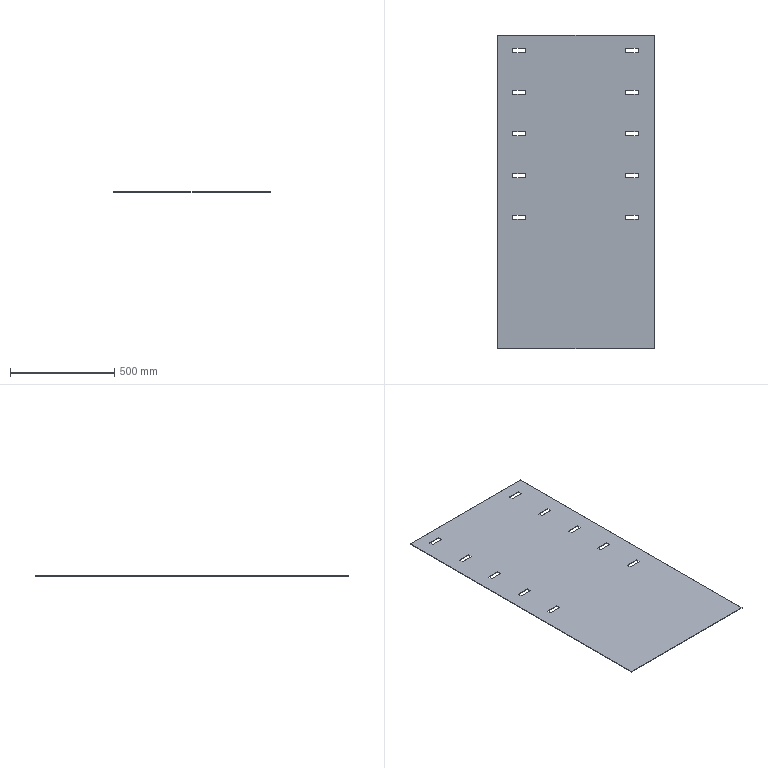Part | SolidWorks | features Cut 1, FlatPattern 1, SMBaseFlange 1, SheetMetal 1 | 1 solid | 46 faces | box 750 x 1500 x 2.5 mm | volume 2781500 mm3 | plane 46
STEP:
#1=CARTESIAN_POINT('',(375.,-750.,0.));
#2=VERTEX_POINT('',#1);
#3=CARTESIAN_POINT('',(375.,750.,0.));
#4=VERTEX_POINT('',#3);
#5=CARTESIAN_POINT('',(375.,750.,0.));
#6=DIRECTION('',(0.,1.,0.));
#7=VECTOR('',#6,1000.);
#8=LINE('',#5,#7);
#9=EDGE_CURVE('',#2,#4,#8,.T.);
#10=ORIENTED_EDGE('',*,*,#9,.F.);
#11=CARTESIAN_POINT('',(375.,-750.,-2.5));
#12=VERTEX_POINT('',#11);
#13=CARTESIAN_POINT('',(375.,-750.,-2.5));
#14=DIRECTION('',(0.,0.,1.));
#15=VECTOR('',#14,1000.);
#16=LINE('',#13,#15);
#17=EDGE_CURVE('',#12,#2,#16,.T.);
#18=ORIENTED_EDGE('',*,*,#17,.F.);
#19=CARTESIAN_POINT('',(375.,750.,-2.5));
#20=VERTEX_POINT('',#19);
#21=CARTESIAN_POINT('',(375.,750.,-2.5));
#22=DIRECTION('',(0.,1.,0.));
#23=VECTOR('',#22,1000.);
#24=LINE('',#21,#23);
#25=EDGE_CURVE('',#12,#20,#24,.T.);
#26=ORIENTED_EDGE('',*,*,#25,.T.);
#27=CARTESIAN_POINT('',(375.,750.,-2.5));
#28=DIRECTION('',(0.,0.,1.));
#29=VECTOR('',#28,1000.);
#30=LINE('',#27,#29);
#31=EDGE_CURVE('',#20,#4,#30,.T.);
#32=ORIENTED_EDGE('',*,*,#31,.T.);
#33=EDGE_LOOP('',(#10,#18,#26,#32));
#34=FACE_OUTER_BOUND('',#33,.T.);
#35=CARTESIAN_POINT('',(375.,750.,-2.5));
#36=DIRECTION('',(1.,0.,0.));
#37=DIRECTION('',(0.,0.,-1.));
#38=AXIS2_PLACEMENT_3D('',#35,#36,#37);
#39=PLANE('',#38);
#40=ADVANCED_FACE('',(#34),#39,.T.);
#41=CARTESIAN_POINT('',(-375.,-750.,0.));
#42=VERTEX_POINT('',#41);
#43=CARTESIAN_POINT('',(-375.,-750.,0.));
#44=DIRECTION('',(1.,0.,0.));
#45=VECTOR('',#44,1000.);
#46=LINE('',#43,#45);
#47=EDGE_CURVE('',#42,#2,#46,.T.);
#48=ORIENTED_EDGE('',*,*,#47,.F.);
#49=CARTESIAN_POINT('',(-375.,-750.,-2.5));
#50=VERTEX_POINT('',#49);
#51=CARTESIAN_POINT('',(-375.,-750.,-2.5));
#52=DIRECTION('',(0.,0.,1.));
#53=VECTOR('',#52,1000.);
#54=LINE('',#51,#53);
#55=EDGE_CURVE('',#50,#42,#54,.T.);
#56=ORIENTED_EDGE('',*,*,#55,.F.);
#57=CARTESIAN_POINT('',(-375.,-750.,-2.5));
#58=DIRECTION('',(1.,0.,0.));
#59=VECTOR('',#58,1000.);
#60=LINE('',#57,#59);
#61=EDGE_CURVE('',#50,#12,#60,.T.);
#62=ORIENTED_EDGE('',*,*,#61,.T.);
#63=ORIENTED_EDGE('',*,*,#17,.T.);
#64=EDGE_LOOP('',(#48,#56,#62,#63));
#65=FACE_OUTER_BOUND('',#64,.T.);
#66=CARTESIAN_POINT('',(-375.,-750.,-2.5));
#67=DIRECTION('',(0.,-1.,0.));
#68=DIRECTION('',(0.,0.,-1.));
#69=AXIS2_PLACEMENT_3D('',#66,#67,#68);
#70=PLANE('',#69);
#71=ADVANCED_FACE('',(#65),#70,.T.);
#72=CARTESIAN_POINT('',(-375.,750.,0.));
#73=VERTEX_POINT('',#72);
#74=CARTESIAN_POINT('',(-375.,750.,0.));
#75=DIRECTION('',(0.,-1.,0.));
#76=VECTOR('',#75,1000.);
#77=LINE('',#74,#76);
#78=EDGE_CURVE('',#73,#42,#77,.T.);
#79=ORIENTED_EDGE('',*,*,#78,.F.);
#80=CARTESIAN_POINT('',(-375.,750.,-2.5));
#81=VERTEX_POINT('',#80);
#82=CARTESIAN_POINT('',(-375.,750.,-2.5));
#83=DIRECTION('',(0.,0.,1.));
#84=VECTOR('',#83,1000.);
#85=LINE('',#82,#84);
#86=EDGE_CURVE('',#81,#73,#85,.T.);
#87=ORIENTED_EDGE('',*,*,#86,.F.);
#88=CARTESIAN_POINT('',(-375.,750.,-2.5));
#89=DIRECTION('',(0.,-1.,0.));
#90=VECTOR('',#89,1000.);
#91=LINE('',#88,#90);
#92=EDGE_CURVE('',#81,#50,#91,.T.);
#93=ORIENTED_EDGE('',*,*,#92,.T.);
#94=ORIENTED_EDGE('',*,*,#55,.T.);
#95=EDGE_LOOP('',(#79,#87,#93,#94));
#96=FACE_OUTER_BOUND('',#95,.T.);
#97=CARTESIAN_POINT('',(-375.,750.,-2.5));
#98=DIRECTION('',(-1.,0.,0.));
#99=DIRECTION('',(0.,0.,1.));
#100=AXIS2_PLACEMENT_3D('',#97,#98,#99);
#101=PLANE('',#100);
#102=ADVANCED_FACE('',(#96),#101,.T.);
#103=CARTESIAN_POINT('',(-375.,750.,0.));
#104=DIRECTION('',(-1.,0.,0.));
#105=VECTOR('',#104,1000.);
#106=LINE('',#103,#105);
#107=EDGE_CURVE('',#4,#73,#106,.T.);
#108=ORIENTED_EDGE('',*,*,#107,.F.);
#109=ORIENTED_EDGE('',*,*,#31,.F.);
#110=CARTESIAN_POINT('',(-375.,750.,-2.5));
#111=DIRECTION('',(-1.,0.,0.));
#112=VECTOR('',#111,1000.);
#113=LINE('',#110,#112);
#114=EDGE_CURVE('',#20,#81,#113,.T.);
#115=ORIENTED_EDGE('',*,*,#114,.T.);
#116=ORIENTED_EDGE('',*,*,#86,.T.);
#117=EDGE_LOOP('',(#108,#109,#115,#116));
#118=FACE_OUTER_BOUND('',#117,.T.);
#119=CARTESIAN_POINT('',(-375.,750.,-2.5));
#120=DIRECTION('',(0.,1.,0.));
#121=DIRECTION('',(0.,0.,1.));
#122=AXIS2_PLACEMENT_3D('',#119,#120,#121);
#123=PLANE('',#122);
#124=ADVANCED_FACE('',(#118),#123,.T.);
#125=CARTESIAN_POINT('',(298.5,-111.5,-2.5));
#126=VERTEX_POINT('',#125);
#127=CARTESIAN_POINT('',(236.5,-111.5,-2.5));
#128=VERTEX_POINT('',#127);
#129=CARTESIAN_POINT('',(236.5,-111.5,-2.5));
#130=DIRECTION('',(-1.,0.,0.));
#131=VECTOR('',#130,1000.);
#132=LINE('',#129,#131);
#133=EDGE_CURVE('',#126,#128,#132,.T.);
#134=ORIENTED_EDGE('',*,*,#133,.T.);
#135=CARTESIAN_POINT('',(236.5,-131.5,-2.5));
#136=VERTEX_POINT('',#135);
#137=CARTESIAN_POINT('',(236.5,-111.5,-2.5));
#138=DIRECTION('',(0.,-1.,0.));
#139=VECTOR('',#138,1000.);
#140=LINE('',#137,#139);
#141=EDGE_CURVE('',#128,#136,#140,.T.);
#142=ORIENTED_EDGE('',*,*,#141,.T.);
#143=CARTESIAN_POINT('',(298.5,-131.5,-2.5));
#144=VERTEX_POINT('',#143);
#145=CARTESIAN_POINT('',(236.5,-131.5,-2.5));
#146=DIRECTION('',(1.,0.,0.));
#147=VECTOR('',#146,1000.);
#148=LINE('',#145,#147);
#149=EDGE_CURVE('',#136,#144,#148,.T.);
#150=ORIENTED_EDGE('',*,*,#149,.T.);
#151=CARTESIAN_POINT('',(298.5,-111.5,-2.5));
#152=DIRECTION('',(0.,1.,0.));
#153=VECTOR('',#152,1000.);
#154=LINE('',#151,#153);
#155=EDGE_CURVE('',#144,#126,#154,.T.);
#156=ORIENTED_EDGE('',*,*,#155,.T.);
#157=EDGE_LOOP('',(#134,#142,#150,#156));
#158=FACE_BOUND('',#157,.T.);
#159=CARTESIAN_POINT('',(-241.5,-111.5,-2.5));
#160=VERTEX_POINT('',#159);
#161=CARTESIAN_POINT('',(-303.5,-111.5,-2.5));
#162=VERTEX_POINT('',#161);
#163=CARTESIAN_POINT('',(-303.5,-111.5,-2.5));
#164=DIRECTION('',(-1.,0.,0.));
#165=VECTOR('',#164,1000.);
#166=LINE('',#163,#165);
#167=EDGE_CURVE('',#160,#162,#166,.T.);
#168=ORIENTED_EDGE('',*,*,#167,.T.);
#169=CARTESIAN_POINT('',(-303.5,-131.5,-2.5));
#170=VERTEX_POINT('',#169);
#171=CARTESIAN_POINT('',(-303.5,-111.5,-2.5));
#172=DIRECTION('',(0.,-1.,0.));
#173=VECTOR('',#172,1000.);
#174=LINE('',#171,#173);
#175=EDGE_CURVE('',#162,#170,#174,.T.);
#176=ORIENTED_EDGE('',*,*,#175,.T.);
#177=CARTESIAN_POINT('',(-241.5,-131.5,-2.5));
#178=VERTEX_POINT('',#177);
#179=CARTESIAN_POINT('',(-303.5,-131.5,-2.5));
#180=DIRECTION('',(1.,0.,0.));
#181=VECTOR('',#180,1000.);
#182=LINE('',#179,#181);
#183=EDGE_CURVE('',#170,#178,#182,.T.);
#184=ORIENTED_EDGE('',*,*,#183,.T.);
#185=CARTESIAN_POINT('',(-241.5,-111.5,-2.5));
#186=DIRECTION('',(0.,1.,0.));
#187=VECTOR('',#186,1000.);
#188=LINE('',#185,#187);
#189=EDGE_CURVE('',#178,#160,#188,.T.);
#190=ORIENTED_EDGE('',*,*,#189,.T.);
#191=EDGE_LOOP('',(#168,#176,#184,#190));
#192=FACE_BOUND('',#191,.T.);
#193=CARTESIAN_POINT('',(298.5,88.5,-2.5));
#194=VERTEX_POINT('',#193);
#195=CARTESIAN_POINT('',(236.5,88.5,-2.5));
#196=VERTEX_POINT('',#195);
#197=CARTESIAN_POINT('',(236.5,88.5,-2.5));
#198=DIRECTION('',(-1.,0.,0.));
#199=VECTOR('',#198,1000.);
#200=LINE('',#197,#199);
#201=EDGE_CURVE('',#194,#196,#200,.T.);
#202=ORIENTED_EDGE('',*,*,#201,.T.);
#203=CARTESIAN_POINT('',(236.5,68.5,-2.5));
#204=VERTEX_POINT('',#203);
#205=CARTESIAN_POINT('',(236.5,88.5,-2.5));
#206=DIRECTION('',(0.,-1.,0.));
#207=VECTOR('',#206,1000.);
#208=LINE('',#205,#207);
#209=EDGE_CURVE('',#196,#204,#208,.T.);
#210=ORIENTED_EDGE('',*,*,#209,.T.);
#211=CARTESIAN_POINT('',(298.5,68.5,-2.5));
#212=VERTEX_POINT('',#211);
#213=CARTESIAN_POINT('',(236.5,68.5,-2.5));
#214=DIRECTION('',(1.,0.,0.));
#215=VECTOR('',#214,1000.);
#216=LINE('',#213,#215);
#217=EDGE_CURVE('',#204,#212,#216,.T.);
#218=ORIENTED_EDGE('',*,*,#217,.T.);
#219=CARTESIAN_POINT('',(298.5,88.5,-2.5));
#220=DIRECTION('',(0.,1.,0.));
#221=VECTOR('',#220,1000.);
#222=LINE('',#219,#221);
#223=EDGE_CURVE('',#212,#194,#222,.T.);
#224=ORIENTED_EDGE('',*,*,#223,.T.);
#225=EDGE_LOOP('',(#202,#210,#218,#224));
#226=FACE_BOUND('',#225,.T.);
#227=CARTESIAN_POINT('',(-241.5,288.5,-2.5));
#228=VERTEX_POINT('',#227);
#229=CARTESIAN_POINT('',(-303.5,288.5,-2.5));
#230=VERTEX_POINT('',#229);
#231=CARTESIAN_POINT('',(-303.5,288.5,-2.5));
#232=DIRECTION('',(-1.,0.,0.));
#233=VECTOR('',#232,1000.);
#234=LINE('',#231,#233);
#235=EDGE_CURVE('',#228,#230,#234,.T.);
#236=ORIENTED_EDGE('',*,*,#235,.T.);
#237=CARTESIAN_POINT('',(-303.5,268.5,-2.5));
#238=VERTEX_POINT('',#237);
#239=CARTESIAN_POINT('',(-303.5,288.5,-2.5));
#240=DIRECTION('',(0.,-1.,0.));
#241=VECTOR('',#240,1000.);
#242=LINE('',#239,#241);
#243=EDGE_CURVE('',#230,#238,#242,.T.);
#244=ORIENTED_EDGE('',*,*,#243,.T.);
#245=CARTESIAN_POINT('',(-241.5,268.5,-2.5));
#246=VERTEX_POINT('',#245);
#247=CARTESIAN_POINT('',(-303.5,268.5,-2.5));
#248=DIRECTION('',(1.,0.,0.));
#249=VECTOR('',#248,1000.);
#250=LINE('',#247,#249);
#251=EDGE_CURVE('',#238,#246,#250,.T.);
#252=ORIENTED_EDGE('',*,*,#251,.T.);
#253=CARTESIAN_POINT('',(-241.5,288.5,-2.5));
#254=DIRECTION('',(0.,1.,0.));
#255=VECTOR('',#254,1000.);
#256=LINE('',#253,#255);
#257=EDGE_CURVE('',#246,#228,#256,.T.);
#258=ORIENTED_EDGE('',*,*,#257,.T.);
#259=EDGE_LOOP('',(#236,#244,#252,#258));
#260=FACE_BOUND('',#259,.T.);
#261=CARTESIAN_POINT('',(-241.5,488.5,-2.5));
#262=VERTEX_POINT('',#261);
#263=CARTESIAN_POINT('',(-303.5,488.5,-2.5));
#264=VERTEX_POINT('',#263);
#265=CARTESIAN_POINT('',(-303.5,488.5,-2.5));
#266=DIRECTION('',(-1.,0.,0.));
#267=VECTOR('',#266,1000.);
#268=LINE('',#265,#267);
#269=EDGE_CURVE('',#262,#264,#268,.T.);
#270=ORIENTED_EDGE('',*,*,#269,.T.);
#271=CARTESIAN_POINT('',(-303.5,468.5,-2.5));
#272=VERTEX_POINT('',#271);
#273=CARTESIAN_POINT('',(-303.5,488.5,-2.5));
#274=DIRECTION('',(0.,-1.,0.));
#275=VECTOR('',#274,1000.);
#276=LINE('',#273,#275);
#277=EDGE_CURVE('',#264,#272,#276,.T.);
#278=ORIENTED_EDGE('',*,*,#277,.T.);
#279=CARTESIAN_POINT('',(-241.5,468.5,-2.5));
#280=VERTEX_POINT('',#279);
#281=CARTESIAN_POINT('',(-303.5,468.5,-2.5));
#282=DIRECTION('',(1.,0.,0.));
#283=VECTOR('',#282,1000.);
#284=LINE('',#281,#283);
#285=EDGE_CURVE('',#272,#280,#284,.T.);
#286=ORIENTED_EDGE('',*,*,#285,.T.);
#287=CARTESIAN_POINT('',(-241.5,488.5,-2.5));
#288=DIRECTION('',(0.,1.,0.));
#289=VECTOR('',#288,1000.);
#290=LINE('',#287,#289);
#291=EDGE_CURVE('',#280,#262,#290,.T.);
#292=ORIENTED_EDGE('',*,*,#291,.T.);
#293=EDGE_LOOP('',(#270,#278,#286,#292));
#294=FACE_BOUND('',#293,.T.);
#295=CARTESIAN_POINT('',(-241.5,88.5,-2.5));
#296=VERTEX_POINT('',#295);
#297=CARTESIAN_POINT('',(-303.5,88.5,-2.5));
#298=VERTEX_POINT('',#297);
#299=CARTESIAN_POINT('',(-303.5,88.5,-2.5));
#300=DIRECTION('',(-1.,0.,0.));
#301=VECTOR('',#300,1000.);
#302=LINE('',#299,#301);
#303=EDGE_CURVE('',#296,#298,#302,.T.);
#304=ORIENTED_EDGE('',*,*,#303,.T.);
#305=CARTESIAN_POINT('',(-303.5,68.5,-2.5));
#306=VERTEX_POINT('',#305);
#307=CARTESIAN_POINT('',(-303.5,88.5,-2.5));
#308=DIRECTION('',(0.,-1.,0.));
#309=VECTOR('',#308,1000.);
#310=LINE('',#307,#309);
#311=EDGE_CURVE('',#298,#306,#310,.T.);
#312=ORIENTED_EDGE('',*,*,#311,.T.);
#313=CARTESIAN_POINT('',(-241.5,68.5,-2.5));
#314=VERTEX_POINT('',#313);
#315=CARTESIAN_POINT('',(-303.5,68.5,-2.5));
#316=DIRECTION('',(1.,0.,0.));
#317=VECTOR('',#316,1000.);
#318=LINE('',#315,#317);
#319=EDGE_CURVE('',#306,#314,#318,.T.);
#320=ORIENTED_EDGE('',*,*,#319,.T.);
#321=CARTESIAN_POINT('',(-241.5,88.5,-2.5));
#322=DIRECTION('',(0.,1.,0.));
#323=VECTOR('',#322,1000.);
#324=LINE('',#321,#323);
#325=EDGE_CURVE('',#314,#296,#324,.T.);
#326=ORIENTED_EDGE('',*,*,#325,.T.);
#327=EDGE_LOOP('',(#304,#312,#320,#326));
#328=FACE_BOUND('',#327,.T.);
#329=CARTESIAN_POINT('',(298.5,688.5,-2.5));
#330=VERTEX_POINT('',#329);
#331=CARTESIAN_POINT('',(236.5,688.5,-2.5));
#332=VERTEX_POINT('',#331);
#333=CARTESIAN_POINT('',(236.5,688.5,-2.5));
#334=DIRECTION('',(-1.,0.,0.));
#335=VECTOR('',#334,1000.);
#336=LINE('',#333,#335);
#337=EDGE_CURVE('',#330,#332,#336,.T.);
#338=ORIENTED_EDGE('',*,*,#337,.T.);
#339=CARTESIAN_POINT('',(236.5,668.5,-2.5));
#340=VERTEX_POINT('',#339);
#341=CARTESIAN_POINT('',(236.5,688.5,-2.5));
#342=DIRECTION('',(0.,-1.,0.));
#343=VECTOR('',#342,1000.);
#344=LINE('',#341,#343);
#345=EDGE_CURVE('',#332,#340,#344,.T.);
#346=ORIENTED_EDGE('',*,*,#345,.T.);
#347=CARTESIAN_POINT('',(298.5,668.5,-2.5));
#348=VERTEX_POINT('',#347);
#349=CARTESIAN_POINT('',(236.5,668.5,-2.5));
#350=DIRECTION('',(1.,0.,0.));
#351=VECTOR('',#350,1000.);
#352=LINE('',#349,#351);
#353=EDGE_CURVE('',#340,#348,#352,.T.);
#354=ORIENTED_EDGE('',*,*,#353,.T.);
#355=CARTESIAN_POINT('',(298.5,688.5,-2.5));
#356=DIRECTION('',(0.,1.,0.));
#357=VECTOR('',#356,1000.);
#358=LINE('',#355,#357);
#359=EDGE_CURVE('',#348,#330,#358,.T.);
#360=ORIENTED_EDGE('',*,*,#359,.T.);
#361=EDGE_LOOP('',(#338,#346,#354,#360));
#362=FACE_BOUND('',#361,.T.);
#363=CARTESIAN_POINT('',(298.5,488.5,-2.5));
#364=VERTEX_POINT('',#363);
#365=CARTESIAN_POINT('',(236.5,488.5,-2.5));
#366=VERTEX_POINT('',#365);
#367=CARTESIAN_POINT('',(236.5,488.5,-2.5));
#368=DIRECTION('',(-1.,0.,0.));
#369=VECTOR('',#368,1000.);
#370=LINE('',#367,#369);
#371=EDGE_CURVE('',#364,#366,#370,.T.);
#372=ORIENTED_EDGE('',*,*,#371,.T.);
#373=CARTESIAN_POINT('',(236.5,468.5,-2.5));
#374=VERTEX_POINT('',#373);
#375=CARTESIAN_POINT('',(236.5,488.5,-2.5));
#376=DIRECTION('',(0.,-1.,0.));
#377=VECTOR('',#376,1000.);
#378=LINE('',#375,#377);
#379=EDGE_CURVE('',#366,#374,#378,.T.);
#380=ORIENTED_EDGE('',*,*,#379,.T.);
#381=CARTESIAN_POINT('',(298.5,468.5,-2.5));
#382=VERTEX_POINT('',#381);
#383=CARTESIAN_POINT('',(236.5,468.5,-2.5));
#384=DIRECTION('',(1.,0.,0.));
#385=VECTOR('',#384,1000.);
#386=LINE('',#383,#385);
#387=EDGE_CURVE('',#374,#382,#386,.T.);
#388=ORIENTED_EDGE('',*,*,#387,.T.);
#389=CARTESIAN_POINT('',(298.5,488.5,-2.5));
#390=DIRECTION('',(0.,1.,0.));
#391=VECTOR('',#390,1000.);
#392=LINE('',#389,#391);
#393=EDGE_CURVE('',#382,#364,#392,.T.);
#394=ORIENTED_EDGE('',*,*,#393,.T.);
#395=EDGE_LOOP('',(#372,#380,#388,#394));
#396=FACE_BOUND('',#395,.T.);
#397=CARTESIAN_POINT('',(298.5,288.5,-2.5));
#398=VERTEX_POINT('',#397);
#399=CARTESIAN_POINT('',(236.5,288.5,-2.5));
#400=VERTEX_POINT('',#399);
#401=CARTESIAN_POINT('',(236.5,288.5,-2.5));
#402=DIRECTION('',(-1.,0.,0.));
#403=VECTOR('',#402,1000.);
#404=LINE('',#401,#403);
#405=EDGE_CURVE('',#398,#400,#404,.T.);
#406=ORIENTED_EDGE('',*,*,#405,.T.);
#407=CARTESIAN_POINT('',(236.5,268.5,-2.5));
#408=VERTEX_POINT('',#407);
#409=CARTESIAN_POINT('',(236.5,288.5,-2.5));
#410=DIRECTION('',(0.,-1.,0.));
#411=VECTOR('',#410,1000.);
#412=LINE('',#409,#411);
#413=EDGE_CURVE('',#400,#408,#412,.T.);
#414=ORIENTED_EDGE('',*,*,#413,.T.);
#415=CARTESIAN_POINT('',(298.5,268.5,-2.5));
#416=VERTEX_POINT('',#415);
#417=CARTESIAN_POINT('',(236.5,268.5,-2.5));
#418=DIRECTION('',(1.,0.,0.));
#419=VECTOR('',#418,1000.);
#420=LINE('',#417,#419);
#421=EDGE_CURVE('',#408,#416,#420,.T.);
#422=ORIENTED_EDGE('',*,*,#421,.T.);
#423=CARTESIAN_POINT('',(298.5,288.5,-2.5));
#424=DIRECTION('',(0.,1.,0.));
#425=VECTOR('',#424,1000.);
#426=LINE('',#423,#425);
#427=EDGE_CURVE('',#416,#398,#426,.T.);
#428=ORIENTED_EDGE('',*,*,#427,.T.);
#429=EDGE_LOOP('',(#406,#414,#422,#428));
#430=FACE_BOUND('',#429,.T.);
#431=CARTESIAN_POINT('',(-241.5,688.5,-2.5));
#432=VERTEX_POINT('',#431);
#433=CARTESIAN_POINT('',(-303.5,688.5,-2.5));
#434=VERTEX_POINT('',#433);
#435=CARTESIAN_POINT('',(-303.5,688.5,-2.5));
#436=DIRECTION('',(-1.,0.,0.));
#437=VECTOR('',#436,1000.);
#438=LINE('',#435,#437);
#439=EDGE_CURVE('',#432,#434,#438,.T.);
#440=ORIENTED_EDGE('',*,*,#439,.T.);
#441=CARTESIAN_POINT('',(-303.5,668.5,-2.5));
#442=VERTEX_POINT('',#441);
#443=CARTESIAN_POINT('',(-303.5,688.5,-2.5));
#444=DIRECTION('',(0.,-1.,0.));
#445=VECTOR('',#444,1000.);
#446=LINE('',#443,#445);
#447=EDGE_CURVE('',#434,#442,#446,.T.);
#448=ORIENTED_EDGE('',*,*,#447,.T.);
#449=CARTESIAN_POINT('',(-241.5,668.5,-2.5));
#450=VERTEX_POINT('',#449);
#451=CARTESIAN_POINT('',(-303.5,668.5,-2.5));
#452=DIRECTION('',(1.,0.,0.));
#453=VECTOR('',#452,1000.);
#454=LINE('',#451,#453);
#455=EDGE_CURVE('',#442,#450,#454,.T.);
#456=ORIENTED_EDGE('',*,*,#455,.T.);
#457=CARTESIAN_POINT('',(-241.5,688.5,-2.5));
#458=DIRECTION('',(0.,1.,0.));
#459=VECTOR('',#458,1000.);
#460=LINE('',#457,#459);
#461=EDGE_CURVE('',#450,#432,#460,.T.);
#462=ORIENTED_EDGE('',*,*,#461,.T.);
#463=EDGE_LOOP('',(#440,#448,#456,#462));
#464=FACE_BOUND('',#463,.T.);
#465=ORIENTED_EDGE('',*,*,#25,.F.);
#466=ORIENTED_EDGE('',*,*,#61,.F.);
#467=ORIENTED_EDGE('',*,*,#92,.F.);
#468=ORIENTED_EDGE('',*,*,#114,.F.);
#469=EDGE_LOOP('',(#465,#466,#467,#468));
#470=FACE_OUTER_BOUND('',#469,.T.);
#471=CARTESIAN_POINT('',(0.,0.,-2.5));
#472=DIRECTION('',(0.,0.,1.));
#473=DIRECTION('',(1.,0.,0.));
#474=AXIS2_PLACEMENT_3D('',#471,#472,#473);
#475=PLANE('',#474);
#476=ADVANCED_FACE('',(#158,#192,#226,#260,#294,#328,#362,#396,#430,#464,#470),#475,.F.);
#477=CARTESIAN_POINT('',(236.5,-111.5,0.));
#478=VERTEX_POINT('',#477);
#479=CARTESIAN_POINT('',(236.5,-131.5,0.));
#480=VERTEX_POINT('',#479);
#481=CARTESIAN_POINT('',(236.5,-111.5,0.));
#482=DIRECTION('',(0.,-1.,0.));
#483=VECTOR('',#482,1000.);
#484=LINE('',#481,#483);
#485=EDGE_CURVE('',#478,#480,#484,.T.);
#486=ORIENTED_EDGE('',*,*,#485,.F.);
#487=CARTESIAN_POINT('',(298.5,-111.5,0.));
#488=VERTEX_POINT('',#487);
#489=CARTESIAN_POINT('',(236.5,-111.5,0.));
#490=DIRECTION('',(-1.,0.,0.));
#491=VECTOR('',#490,1000.);
#492=LINE('',#489,#491);
#493=EDGE_CURVE('',#488,#478,#492,.T.);
#494=ORIENTED_EDGE('',*,*,#493,.F.);
#495=CARTESIAN_POINT('',(298.5,-131.5,0.));
#496=VERTEX_POINT('',#495);
#497=CARTESIAN_POINT('',(298.5,-111.5,0.));
#498=DIRECTION('',(0.,1.,0.));
#499=VECTOR('',#498,1000.);
#500=LINE('',#497,#499);
#501=EDGE_CURVE('',#496,#488,#500,.T.);
#502=ORIENTED_EDGE('',*,*,#501,.F.);
#503=CARTESIAN_POINT('',(236.5,-131.5,0.));
#504=DIRECTION('',(1.,0.,0.));
#505=VECTOR('',#504,1000.);
#506=LINE('',#503,#505);
#507=EDGE_CURVE('',#480,#496,#506,.T.);
#508=ORIENTED_EDGE('',*,*,#507,.F.);
#509=EDGE_LOOP('',(#486,#494,#502,#508));
#510=FACE_BOUND('',#509,.T.);
#511=CARTESIAN_POINT('',(-303.5,-111.5,0.));
#512=VERTEX_POINT('',#511);
#513=CARTESIAN_POINT('',(-303.5,-131.5,0.));
#514=VERTEX_POINT('',#513);
#515=CARTESIAN_POINT('',(-303.5,-111.5,0.));
#516=DIRECTION('',(0.,-1.,0.));
#517=VECTOR('',#516,1000.);
#518=LINE('',#515,#517);
#519=EDGE_CURVE('',#512,#514,#518,.T.);
#520=ORIENTED_EDGE('',*,*,#519,.F.);
#521=CARTESIAN_POINT('',(-241.5,-111.5,0.));
#522=VERTEX_POINT('',#521);
#523=CARTESIAN_POINT('',(-303.5,-111.5,0.));
#524=DIRECTION('',(-1.,0.,0.));
#525=VECTOR('',#524,1000.);
#526=LINE('',#523,#525);
#527=EDGE_CURVE('',#522,#512,#526,.T.);
#528=ORIENTED_EDGE('',*,*,#527,.F.);
#529=CARTESIAN_POINT('',(-241.5,-131.5,0.));
#530=VERTEX_POINT('',#529);
#531=CARTESIAN_POINT('',(-241.5,-111.5,0.));
#532=DIRECTION('',(0.,1.,0.));
#533=VECTOR('',#532,1000.);
#534=LINE('',#531,#533);
#535=EDGE_CURVE('',#530,#522,#534,.T.);
#536=ORIENTED_EDGE('',*,*,#535,.F.);
#537=CARTESIAN_POINT('',(-303.5,-131.5,0.));
#538=DIRECTION('',(1.,0.,0.));
#539=VECTOR('',#538,1000.);
#540=LINE('',#537,#539);
#541=EDGE_CURVE('',#514,#530,#540,.T.);
#542=ORIENTED_EDGE('',*,*,#541,.F.);
#543=EDGE_LOOP('',(#520,#528,#536,#542));
#544=FACE_BOUND('',#543,.T.);
#545=CARTESIAN_POINT('',(236.5,88.5,0.));
#546=VERTEX_POINT('',#545);
#547=CARTESIAN_POINT('',(236.5,68.5,0.));
#548=VERTEX_POINT('',#547);
#549=CARTESIAN_POINT('',(236.5,88.5,0.));
#550=DIRECTION('',(0.,-1.,0.));
#551=VECTOR('',#550,1000.);
#552=LINE('',#549,#551);
#553=EDGE_CURVE('',#546,#548,#552,.T.);
#554=ORIENTED_EDGE('',*,*,#553,.F.);
#555=CARTESIAN_POINT('',(298.5,88.5,0.));
#556=VERTEX_POINT('',#555);
#557=CARTESIAN_POINT('',(236.5,88.5,0.));
#558=DIRECTION('',(-1.,0.,0.));
#559=VECTOR('',#558,1000.);
#560=LINE('',#557,#559);
#561=EDGE_CURVE('',#556,#546,#560,.T.);
#562=ORIENTED_EDGE('',*,*,#561,.F.);
#563=CARTESIAN_POINT('',(298.5,68.5,0.));
#564=VERTEX_POINT('',#563);
#565=CARTESIAN_POINT('',(298.5,88.5,0.));
#566=DIRECTION('',(0.,1.,0.));
#567=VECTOR('',#566,1000.);
#568=LINE('',#565,#567);
#569=EDGE_CURVE('',#564,#556,#568,.T.);
#570=ORIENTED_EDGE('',*,*,#569,.F.);
#571=CARTESIAN_POINT('',(236.5,68.5,0.));
#572=DIRECTION('',(1.,0.,0.));
#573=VECTOR('',#572,1000.);
#574=LINE('',#571,#573);
#575=EDGE_CURVE('',#548,#564,#574,.T.);
#576=ORIENTED_EDGE('',*,*,#575,.F.);
#577=EDGE_LOOP('',(#554,#562,#570,#576));
#578=FACE_BOUND('',#577,.T.);
#579=CARTESIAN_POINT('',(-303.5,288.5,0.));
#580=VERTEX_POINT('',#579);
#581=CARTESIAN_POINT('',(-303.5,268.5,0.));
#582=VERTEX_POINT('',#581);
#583=CARTESIAN_POINT('',(-303.5,288.5,0.));
#584=DIRECTION('',(0.,-1.,0.));
#585=VECTOR('',#584,1000.);
#586=LINE('',#583,#585);
#587=EDGE_CURVE('',#580,#582,#586,.T.);
#588=ORIENTED_EDGE('',*,*,#587,.F.);
#589=CARTESIAN_POINT('',(-241.5,288.5,0.));
#590=VERTEX_POINT('',#589);
#591=CARTESIAN_POINT('',(-303.5,288.5,0.));
#592=DIRECTION('',(-1.,0.,0.));
#593=VECTOR('',#592,1000.);
#594=LINE('',#591,#593);
#595=EDGE_CURVE('',#590,#580,#594,.T.);
#596=ORIENTED_EDGE('',*,*,#595,.F.);
#597=CARTESIAN_POINT('',(-241.5,268.5,0.));
#598=VERTEX_POINT('',#597);
#599=CARTESIAN_POINT('',(-241.5,288.5,0.));
#600=DIRECTION('',(0.,1.,0.));
#601=VECTOR('',#600,1000.);
#602=LINE('',#599,#601);
#603=EDGE_CURVE('',#598,#590,#602,.T.);
#604=ORIENTED_EDGE('',*,*,#603,.F.);
#605=CARTESIAN_POINT('',(-303.5,268.5,0.));
#606=DIRECTION('',(1.,0.,0.));
#607=VECTOR('',#606,1000.);
#608=LINE('',#605,#607);
#609=EDGE_CURVE('',#582,#598,#608,.T.);
#610=ORIENTED_EDGE('',*,*,#609,.F.);
#611=EDGE_LOOP('',(#588,#596,#604,#610));
#612=FACE_BOUND('',#611,.T.);
#613=CARTESIAN_POINT('',(-303.5,488.5,0.));
#614=VERTEX_POINT('',#613);
#615=CARTESIAN_POINT('',(-303.5,468.5,0.));
#616=VERTEX_POINT('',#615);
#617=CARTESIAN_POINT('',(-303.5,488.5,0.));
#618=DIRECTION('',(0.,-1.,0.));
#619=VECTOR('',#618,1000.);
#620=LINE('',#617,#619);
#621=EDGE_CURVE('',#614,#616,#620,.T.);
#622=ORIENTED_EDGE('',*,*,#621,.F.);
#623=CARTESIAN_POINT('',(-241.5,488.5,0.));
#624=VERTEX_POINT('',#623);
#625=CARTESIAN_POINT('',(-303.5,488.5,0.));
#626=DIRECTION('',(-1.,0.,0.));
#627=VECTOR('',#626,1000.);
#628=LINE('',#625,#627);
#629=EDGE_CURVE('',#624,#614,#628,.T.);
#630=ORIENTED_EDGE('',*,*,#629,.F.);
#631=CARTESIAN_POINT('',(-241.5,468.5,0.));
#632=VERTEX_POINT('',#631);
#633=CARTESIAN_POINT('',(-241.5,488.5,0.));
#634=DIRECTION('',(0.,1.,0.));
#635=VECTOR('',#634,1000.);
#636=LINE('',#633,#635);
#637=EDGE_CURVE('',#632,#624,#636,.T.);
#638=ORIENTED_EDGE('',*,*,#637,.F.);
#639=CARTESIAN_POINT('',(-303.5,468.5,0.));
#640=DIRECTION('',(1.,0.,0.));
#641=VECTOR('',#640,1000.);
#642=LINE('',#639,#641);
#643=EDGE_CURVE('',#616,#632,#642,.T.);
#644=ORIENTED_EDGE('',*,*,#643,.F.);
#645=EDGE_LOOP('',(#622,#630,#638,#644));
#646=FACE_BOUND('',#645,.T.);
#647=CARTESIAN_POINT('',(-303.5,88.5,0.));
#648=VERTEX_POINT('',#647);
#649=CARTESIAN_POINT('',(-303.5,68.5,0.));
#650=VERTEX_POINT('',#649);
#651=CARTESIAN_POINT('',(-303.5,88.5,0.));
#652=DIRECTION('',(0.,-1.,0.));
#653=VECTOR('',#652,1000.);
#654=LINE('',#651,#653);
#655=EDGE_CURVE('',#648,#650,#654,.T.);
#656=ORIENTED_EDGE('',*,*,#655,.F.);
#657=CARTESIAN_POINT('',(-241.5,88.5,0.));
#658=VERTEX_POINT('',#657);
#659=CARTESIAN_POINT('',(-303.5,88.5,0.));
#660=DIRECTION('',(-1.,0.,0.));
#661=VECTOR('',#660,1000.);
#662=LINE('',#659,#661);
#663=EDGE_CURVE('',#658,#648,#662,.T.);
#664=ORIENTED_EDGE('',*,*,#663,.F.);
#665=CARTESIAN_POINT('',(-241.5,68.5,0.));
#666=VERTEX_POINT('',#665);
#667=CARTESIAN_POINT('',(-241.5,88.5,0.));
#668=DIRECTION('',(0.,1.,0.));
#669=VECTOR('',#668,1000.);
#670=LINE('',#667,#669);
#671=EDGE_CURVE('',#666,#658,#670,.T.);
#672=ORIENTED_EDGE('',*,*,#671,.F.);
#673=CARTESIAN_POINT('',(-303.5,68.5,0.));
#674=DIRECTION('',(1.,0.,0.));
#675=VECTOR('',#674,1000.);
#676=LINE('',#673,#675);
#677=EDGE_CURVE('',#650,#666,#676,.T.);
#678=ORIENTED_EDGE('',*,*,#677,.F.);
#679=EDGE_LOOP('',(#656,#664,#672,#678));
#680=FACE_BOUND('',#679,.T.);
#681=CARTESIAN_POINT('',(236.5,688.5,0.));
#682=VERTEX_POINT('',#681);
#683=CARTESIAN_POINT('',(236.5,668.5,0.));
#684=VERTEX_POINT('',#683);
#685=CARTESIAN_POINT('',(236.5,688.5,0.));
#686=DIRECTION('',(0.,-1.,0.));
#687=VECTOR('',#686,1000.);
#688=LINE('',#685,#687);
#689=EDGE_CURVE('',#682,#684,#688,.T.);
#690=ORIENTED_EDGE('',*,*,#689,.F.);
#691=CARTESIAN_POINT('',(298.5,688.5,0.));
#692=VERTEX_POINT('',#691);
#693=CARTESIAN_POINT('',(236.5,688.5,0.));
#694=DIRECTION('',(-1.,0.,0.));
#695=VECTOR('',#694,1000.);
#696=LINE('',#693,#695);
#697=EDGE_CURVE('',#692,#682,#696,.T.);
#698=ORIENTED_EDGE('',*,*,#697,.F.);
#699=CARTESIAN_POINT('',(298.5,668.5,0.));
#700=VERTEX_POINT('',#699);
#701=CARTESIAN_POINT('',(298.5,688.5,0.));
#702=DIRECTION('',(0.,1.,0.));
#703=VECTOR('',#702,1000.);
#704=LINE('',#701,#703);
#705=EDGE_CURVE('',#700,#692,#704,.T.);
#706=ORIENTED_EDGE('',*,*,#705,.F.);
#707=CARTESIAN_POINT('',(236.5,668.5,0.));
#708=DIRECTION('',(1.,0.,0.));
#709=VECTOR('',#708,1000.);
#710=LINE('',#707,#709);
#711=EDGE_CURVE('',#684,#700,#710,.T.);
#712=ORIENTED_EDGE('',*,*,#711,.F.);
#713=EDGE_LOOP('',(#690,#698,#706,#712));
#714=FACE_BOUND('',#713,.T.);
#715=CARTESIAN_POINT('',(236.5,488.5,0.));
#716=VERTEX_POINT('',#715);
#717=CARTESIAN_POINT('',(236.5,468.5,0.));
#718=VERTEX_POINT('',#717);
#719=CARTESIAN_POINT('',(236.5,488.5,0.));
#720=DIRECTION('',(0.,-1.,0.));
#721=VECTOR('',#720,1000.);
#722=LINE('',#719,#721);
#723=EDGE_CURVE('',#716,#718,#722,.T.);
#724=ORIENTED_EDGE('',*,*,#723,.F.);
#725=CARTESIAN_POINT('',(298.5,488.5,0.));
#726=VERTEX_POINT('',#725);
#727=CARTESIAN_POINT('',(236.5,488.5,0.));
#728=DIRECTION('',(-1.,0.,0.));
#729=VECTOR('',#728,1000.);
#730=LINE('',#727,#729);
#731=EDGE_CURVE('',#726,#716,#730,.T.);
#732=ORIENTED_EDGE('',*,*,#731,.F.);
#733=CARTESIAN_POINT('',(298.5,468.5,0.));
#734=VERTEX_POINT('',#733);
#735=CARTESIAN_POINT('',(298.5,488.5,0.));
#736=DIRECTION('',(0.,1.,0.));
#737=VECTOR('',#736,1000.);
#738=LINE('',#735,#737);
#739=EDGE_CURVE('',#734,#726,#738,.T.);
#740=ORIENTED_EDGE('',*,*,#739,.F.);
#741=CARTESIAN_POINT('',(236.5,468.5,0.));
#742=DIRECTION('',(1.,0.,0.));
#743=VECTOR('',#742,1000.);
#744=LINE('',#741,#743);
#745=EDGE_CURVE('',#718,#734,#744,.T.);
#746=ORIENTED_EDGE('',*,*,#745,.F.);
#747=EDGE_LOOP('',(#724,#732,#740,#746));
#748=FACE_BOUND('',#747,.T.);
#749=CARTESIAN_POINT('',(236.5,288.5,0.));
#750=VERTEX_POINT('',#749);
#751=CARTESIAN_POINT('',(236.5,268.5,0.));
#752=VERTEX_POINT('',#751);
#753=CARTESIAN_POINT('',(236.5,288.5,0.));
#754=DIRECTION('',(0.,-1.,0.));
#755=VECTOR('',#754,1000.);
#756=LINE('',#753,#755);
#757=EDGE_CURVE('',#750,#752,#756,.T.);
#758=ORIENTED_EDGE('',*,*,#757,.F.);
#759=CARTESIAN_POINT('',(298.5,288.5,0.));
#760=VERTEX_POINT('',#759);
#761=CARTESIAN_POINT('',(236.5,288.5,0.));
#762=DIRECTION('',(-1.,0.,0.));
#763=VECTOR('',#762,1000.);
#764=LINE('',#761,#763);
#765=EDGE_CURVE('',#760,#750,#764,.T.);
#766=ORIENTED_EDGE('',*,*,#765,.F.);
#767=CARTESIAN_POINT('',(298.5,268.5,0.));
#768=VERTEX_POINT('',#767);
#769=CARTESIAN_POINT('',(298.5,288.5,0.));
#770=DIRECTION('',(0.,1.,0.));
#771=VECTOR('',#770,1000.);
#772=LINE('',#769,#771);
#773=EDGE_CURVE('',#768,#760,#772,.T.);
#774=ORIENTED_EDGE('',*,*,#773,.F.);
#775=CARTESIAN_POINT('',(236.5,268.5,0.));
#776=DIRECTION('',(1.,0.,0.));
#777=VECTOR('',#776,1000.);
#778=LINE('',#775,#777);
#779=EDGE_CURVE('',#752,#768,#778,.T.);
#780=ORIENTED_EDGE('',*,*,#779,.F.);
#781=EDGE_LOOP('',(#758,#766,#774,#780));
#782=FACE_BOUND('',#781,.T.);
#783=CARTESIAN_POINT('',(-303.5,688.5,0.));
#784=VERTEX_POINT('',#783);
#785=CARTESIAN_POINT('',(-303.5,668.5,0.));
#786=VERTEX_POINT('',#785);
#787=CARTESIAN_POINT('',(-303.5,688.5,0.));
#788=DIRECTION('',(0.,-1.,0.));
#789=VECTOR('',#788,1000.);
#790=LINE('',#787,#789);
#791=EDGE_CURVE('',#784,#786,#790,.T.);
#792=ORIENTED_EDGE('',*,*,#791,.F.);
#793=CARTESIAN_POINT('',(-241.5,688.5,0.));
#794=VERTEX_POINT('',#793);
#795=CARTESIAN_POINT('',(-303.5,688.5,0.));
#796=DIRECTION('',(-1.,0.,0.));
#797=VECTOR('',#796,1000.);
#798=LINE('',#795,#797);
#799=EDGE_CURVE('',#794,#784,#798,.T.);
#800=ORIENTED_EDGE('',*,*,#799,.F.);
#801=CARTESIAN_POINT('',(-241.5,668.5,0.));
#802=VERTEX_POINT('',#801);
#803=CARTESIAN_POINT('',(-241.5,688.5,0.));
#804=DIRECTION('',(0.,1.,0.));
#805=VECTOR('',#804,1000.);
#806=LINE('',#803,#805);
#807=EDGE_CURVE('',#802,#794,#806,.T.);
#808=ORIENTED_EDGE('',*,*,#807,.F.);
#809=CARTESIAN_POINT('',(-303.5,668.5,0.));
#810=DIRECTION('',(1.,0.,0.));
#811=VECTOR('',#810,1000.);
#812=LINE('',#809,#811);
#813=EDGE_CURVE('',#786,#802,#812,.T.);
#814=ORIENTED_EDGE('',*,*,#813,.F.);
#815=EDGE_LOOP('',(#792,#800,#808,#814));
#816=FACE_BOUND('',#815,.T.);
#817=ORIENTED_EDGE('',*,*,#9,.T.);
#818=ORIENTED_EDGE('',*,*,#107,.T.);
#819=ORIENTED_EDGE('',*,*,#78,.T.);
#820=ORIENTED_EDGE('',*,*,#47,.T.);
#821=EDGE_LOOP('',(#817,#818,#819,#820));
#822=FACE_OUTER_BOUND('',#821,.T.);
#823=CARTESIAN_POINT('',(0.,0.,0.));
#824=DIRECTION('',(0.,0.,1.));
#825=DIRECTION('',(1.,0.,0.));
#826=AXIS2_PLACEMENT_3D('',#823,#824,#825);
#827=PLANE('',#826);
#828=ADVANCED_FACE('',(#510,#544,#578,#612,#646,#680,#714,#748,#782,#816,#822),#827,.T.);
#829=ORIENTED_EDGE('',*,*,#791,.T.);
#830=CARTESIAN_POINT('',(-303.5,668.5,-2.5));
#831=DIRECTION('',(0.,0.,1.));
#832=VECTOR('',#831,1000.);
#833=LINE('',#830,#832);
#834=EDGE_CURVE('',#442,#786,#833,.T.);
#835=ORIENTED_EDGE('',*,*,#834,.F.);
#836=ORIENTED_EDGE('',*,*,#447,.F.);
#837=CARTESIAN_POINT('',(-303.5,688.5,-2.5));
#838=DIRECTION('',(0.,0.,1.));
#839=VECTOR('',#838,1000.);
#840=LINE('',#837,#839);
#841=EDGE_CURVE('',#434,#784,#840,.T.);
#842=ORIENTED_EDGE('',*,*,#841,.T.);
#843=EDGE_LOOP('',(#829,#835,#836,#842));
#844=FACE_OUTER_BOUND('',#843,.T.);
#845=CARTESIAN_POINT('',(-303.5,688.5,-2.5));
#846=DIRECTION('',(-1.,0.,0.));
#847=DIRECTION('',(0.,0.,1.));
#848=AXIS2_PLACEMENT_3D('',#845,#846,#847);
#849=PLANE('',#848);
#850=ADVANCED_FACE('',(#844),#849,.F.);
#851=ORIENTED_EDGE('',*,*,#799,.T.);
#852=ORIENTED_EDGE('',*,*,#841,.F.);
#853=ORIENTED_EDGE('',*,*,#439,.F.);
#854=CARTESIAN_POINT('',(-241.5,688.5,-2.5));
#855=DIRECTION('',(0.,0.,1.));
#856=VECTOR('',#855,1000.);
#857=LINE('',#854,#856);
#858=EDGE_CURVE('',#432,#794,#857,.T.);
#859=ORIENTED_EDGE('',*,*,#858,.T.);
#860=EDGE_LOOP('',(#851,#852,#853,#859));
#861=FACE_OUTER_BOUND('',#860,.T.);
#862=CARTESIAN_POINT('',(-303.5,688.5,-2.5));
#863=DIRECTION('',(0.,1.,0.));
#864=DIRECTION('',(-1.,0.,0.));
#865=AXIS2_PLACEMENT_3D('',#862,#863,#864);
#866=PLANE('',#865);
#867=ADVANCED_FACE('',(#861),#866,.F.);
#868=ORIENTED_EDGE('',*,*,#807,.T.);
#869=ORIENTED_EDGE('',*,*,#858,.F.);
#870=ORIENTED_EDGE('',*,*,#461,.F.);
#871=CARTESIAN_POINT('',(-241.5,668.5,-2.5));
#872=DIRECTION('',(0.,0.,1.));
#873=VECTOR('',#872,1000.);
#874=LINE('',#871,#873);
#875=EDGE_CURVE('',#450,#802,#874,.T.);
#876=ORIENTED_EDGE('',*,*,#875,.T.);
#877=EDGE_LOOP('',(#868,#869,#870,#876));
#878=FACE_OUTER_BOUND('',#877,.T.);
#879=CARTESIAN_POINT('',(-241.5,688.5,-2.5));
#880=DIRECTION('',(1.,0.,0.));
#881=DIRECTION('',(0.,0.,-1.));
#882=AXIS2_PLACEMENT_3D('',#879,#880,#881);
#883=PLANE('',#882);
#884=ADVANCED_FACE('',(#878),#883,.F.);
#885=ORIENTED_EDGE('',*,*,#813,.T.);
#886=ORIENTED_EDGE('',*,*,#875,.F.);
#887=ORIENTED_EDGE('',*,*,#455,.F.);
#888=ORIENTED_EDGE('',*,*,#834,.T.);
#889=EDGE_LOOP('',(#885,#886,#887,#888));
#890=FACE_OUTER_BOUND('',#889,.T.);
#891=CARTESIAN_POINT('',(-303.5,668.5,-2.5));
#892=DIRECTION('',(0.,-1.,0.));
#893=DIRECTION('',(0.,0.,-1.));
#894=AXIS2_PLACEMENT_3D('',#891,#892,#893);
#895=PLANE('',#894);
#896=ADVANCED_FACE('',(#890),#895,.F.);
#897=ORIENTED_EDGE('',*,*,#757,.T.);
#898=CARTESIAN_POINT('',(236.5,268.5,-2.5));
#899=DIRECTION('',(0.,0.,1.));
#900=VECTOR('',#899,1000.);
#901=LINE('',#898,#900);
#902=EDGE_CURVE('',#408,#752,#901,.T.);
#903=ORIENTED_EDGE('',*,*,#902,.F.);
#904=ORIENTED_EDGE('',*,*,#413,.F.);
#905=CARTESIAN_POINT('',(236.5,288.5,-2.5));
#906=DIRECTION('',(0.,0.,1.));
#907=VECTOR('',#906,1000.);
#908=LINE('',#905,#907);
#909=EDGE_CURVE('',#400,#750,#908,.T.);
#910=ORIENTED_EDGE('',*,*,#909,.T.);
#911=EDGE_LOOP('',(#897,#903,#904,#910));
#912=FACE_OUTER_BOUND('',#911,.T.);
#913=CARTESIAN_POINT('',(236.5,288.5,-2.5));
#914=DIRECTION('',(-1.,0.,0.));
#915=DIRECTION('',(0.,0.,1.));
#916=AXIS2_PLACEMENT_3D('',#913,#914,#915);
#917=PLANE('',#916);
#918=ADVANCED_FACE('',(#912),#917,.F.);
#919=ORIENTED_EDGE('',*,*,#765,.T.);
#920=ORIENTED_EDGE('',*,*,#909,.F.);
#921=ORIENTED_EDGE('',*,*,#405,.F.);
#922=CARTESIAN_POINT('',(298.5,288.5,-2.5));
#923=DIRECTION('',(0.,0.,1.));
#924=VECTOR('',#923,1000.);
#925=LINE('',#922,#924);
#926=EDGE_CURVE('',#398,#760,#925,.T.);
#927=ORIENTED_EDGE('',*,*,#926,.T.);
#928=EDGE_LOOP('',(#919,#920,#921,#927));
#929=FACE_OUTER_BOUND('',#928,.T.);
#930=CARTESIAN_POINT('',(236.5,288.5,-2.5));
#931=DIRECTION('',(0.,1.,0.));
#932=DIRECTION('',(-1.,0.,0.));
#933=AXIS2_PLACEMENT_3D('',#930,#931,#932);
#934=PLANE('',#933);
#935=ADVANCED_FACE('',(#929),#934,.F.);
#936=ORIENTED_EDGE('',*,*,#773,.T.);
#937=ORIENTED_EDGE('',*,*,#926,.F.);
#938=ORIENTED_EDGE('',*,*,#427,.F.);
#939=CARTESIAN_POINT('',(298.5,268.5,-2.5));
#940=DIRECTION('',(0.,0.,1.));
#941=VECTOR('',#940,1000.);
#942=LINE('',#939,#941);
#943=EDGE_CURVE('',#416,#768,#942,.T.);
#944=ORIENTED_EDGE('',*,*,#943,.T.);
#945=EDGE_LOOP('',(#936,#937,#938,#944));
#946=FACE_OUTER_BOUND('',#945,.T.);
#947=CARTESIAN_POINT('',(298.5,288.5,-2.5));
#948=DIRECTION('',(1.,0.,0.));
#949=DIRECTION('',(0.,0.,-1.));
#950=AXIS2_PLACEMENT_3D('',#947,#948,#949);
#951=PLANE('',#950);
#952=ADVANCED_FACE('',(#946),#951,.F.);
#953=ORIENTED_EDGE('',*,*,#779,.T.);
#954=ORIENTED_EDGE('',*,*,#943,.F.);
#955=ORIENTED_EDGE('',*,*,#421,.F.);
#956=ORIENTED_EDGE('',*,*,#902,.T.);
#957=EDGE_LOOP('',(#953,#954,#955,#956));
#958=FACE_OUTER_BOUND('',#957,.T.);
#959=CARTESIAN_POINT('',(236.5,268.5,-2.5));
#960=DIRECTION('',(0.,-1.,0.));
#961=DIRECTION('',(0.,0.,-1.));
#962=AXIS2_PLACEMENT_3D('',#959,#960,#961);
#963=PLANE('',#962);
#964=ADVANCED_FACE('',(#958),#963,.F.);
#965=ORIENTED_EDGE('',*,*,#723,.T.);
#966=CARTESIAN_POINT('',(236.5,468.5,-2.5));
#967=DIRECTION('',(0.,0.,1.));
#968=VECTOR('',#967,1000.);
#969=LINE('',#966,#968);
#970=EDGE_CURVE('',#374,#718,#969,.T.);
#971=ORIENTED_EDGE('',*,*,#970,.F.);
#972=ORIENTED_EDGE('',*,*,#379,.F.);
#973=CARTESIAN_POINT('',(236.5,488.5,-2.5));
#974=DIRECTION('',(0.,0.,1.));
#975=VECTOR('',#974,1000.);
#976=LINE('',#973,#975);
#977=EDGE_CURVE('',#366,#716,#976,.T.);
#978=ORIENTED_EDGE('',*,*,#977,.T.);
#979=EDGE_LOOP('',(#965,#971,#972,#978));
#980=FACE_OUTER_BOUND('',#979,.T.);
#981=CARTESIAN_POINT('',(236.5,488.5,-2.5));
#982=DIRECTION('',(-1.,0.,0.));
#983=DIRECTION('',(0.,0.,1.));
#984=AXIS2_PLACEMENT_3D('',#981,#982,#983);
#985=PLANE('',#984);
#986=ADVANCED_FACE('',(#980),#985,.F.);
#987=ORIENTED_EDGE('',*,*,#731,.T.);
#988=ORIENTED_EDGE('',*,*,#977,.F.);
#989=ORIENTED_EDGE('',*,*,#371,.F.);
#990=CARTESIAN_POINT('',(298.5,488.5,-2.5));
#991=DIRECTION('',(0.,0.,1.));
#992=VECTOR('',#991,1000.);
#993=LINE('',#990,#992);
#994=EDGE_CURVE('',#364,#726,#993,.T.);
#995=ORIENTED_EDGE('',*,*,#994,.T.);
#996=EDGE_LOOP('',(#987,#988,#989,#995));
#997=FACE_OUTER_BOUND('',#996,.T.);
#998=CARTESIAN_POINT('',(236.5,488.5,-2.5));
#999=DIRECTION('',(0.,1.,0.));
#1000=DIRECTION('',(-1.,0.,0.));
#1001=AXIS2_PLACEMENT_3D('',#998,#999,#1000);
#1002=PLANE('',#1001);
#1003=ADVANCED_FACE('',(#997),#1002,.F.);
#1004=ORIENTED_EDGE('',*,*,#739,.T.);
#1005=ORIENTED_EDGE('',*,*,#994,.F.);
#1006=ORIENTED_EDGE('',*,*,#393,.F.);
#1007=CARTESIAN_POINT('',(298.5,468.5,-2.5));
#1008=DIRECTION('',(0.,0.,1.));
#1009=VECTOR('',#1008,1000.);
#1010=LINE('',#1007,#1009);
#1011=EDGE_CURVE('',#382,#734,#1010,.T.);
#1012=ORIENTED_EDGE('',*,*,#1011,.T.);
#1013=EDGE_LOOP('',(#1004,#1005,#1006,#1012));
#1014=FACE_OUTER_BOUND('',#1013,.T.);
#1015=CARTESIAN_POINT('',(298.5,488.5,-2.5));
#1016=DIRECTION('',(1.,0.,0.));
#1017=DIRECTION('',(0.,0.,-1.));
#1018=AXIS2_PLACEMENT_3D('',#1015,#1016,#1017);
#1019=PLANE('',#1018);
#1020=ADVANCED_FACE('',(#1014),#1019,.F.);
#1021=ORIENTED_EDGE('',*,*,#745,.T.);
#1022=ORIENTED_EDGE('',*,*,#1011,.F.);
#1023=ORIENTED_EDGE('',*,*,#387,.F.);
#1024=ORIENTED_EDGE('',*,*,#970,.T.);
#1025=EDGE_LOOP('',(#1021,#1022,#1023,#1024));
#1026=FACE_OUTER_BOUND('',#1025,.T.);
#1027=CARTESIAN_POINT('',(236.5,468.5,-2.5));
#1028=DIRECTION('',(0.,-1.,0.));
#1029=DIRECTION('',(0.,0.,-1.));
#1030=AXIS2_PLACEMENT_3D('',#1027,#1028,#1029);
#1031=PLANE('',#1030);
#1032=ADVANCED_FACE('',(#1026),#1031,.F.);
#1033=ORIENTED_EDGE('',*,*,#689,.T.);
#1034=CARTESIAN_POINT('',(236.5,668.5,-2.5));
#1035=DIRECTION('',(0.,0.,1.));
#1036=VECTOR('',#1035,1000.);
#1037=LINE('',#1034,#1036);
#1038=EDGE_CURVE('',#340,#684,#1037,.T.);
#1039=ORIENTED_EDGE('',*,*,#1038,.F.);
#1040=ORIENTED_EDGE('',*,*,#345,.F.);
#1041=CARTESIAN_POINT('',(236.5,688.5,-2.5));
#1042=DIRECTION('',(0.,0.,1.));
#1043=VECTOR('',#1042,1000.);
#1044=LINE('',#1041,#1043);
#1045=EDGE_CURVE('',#332,#682,#1044,.T.);
#1046=ORIENTED_EDGE('',*,*,#1045,.T.);
#1047=EDGE_LOOP('',(#1033,#1039,#1040,#1046));
#1048=FACE_OUTER_BOUND('',#1047,.T.);
#1049=CARTESIAN_POINT('',(236.5,688.5,-2.5));
#1050=DIRECTION('',(-1.,0.,0.));
#1051=DIRECTION('',(0.,0.,1.));
#1052=AXIS2_PLACEMENT_3D('',#1049,#1050,#1051);
#1053=PLANE('',#1052);
#1054=ADVANCED_FACE('',(#1048),#1053,.F.);
#1055=ORIENTED_EDGE('',*,*,#697,.T.);
#1056=ORIENTED_EDGE('',*,*,#1045,.F.);
#1057=ORIENTED_EDGE('',*,*,#337,.F.);
#1058=CARTESIAN_POINT('',(298.5,688.5,-2.5));
#1059=DIRECTION('',(0.,0.,1.));
#1060=VECTOR('',#1059,1000.);
#1061=LINE('',#1058,#1060);
#1062=EDGE_CURVE('',#330,#692,#1061,.T.);
#1063=ORIENTED_EDGE('',*,*,#1062,.T.);
#1064=EDGE_LOOP('',(#1055,#1056,#1057,#1063));
#1065=FACE_OUTER_BOUND('',#1064,.T.);
#1066=CARTESIAN_POINT('',(236.5,688.5,-2.5));
#1067=DIRECTION('',(0.,1.,0.));
#1068=DIRECTION('',(-1.,0.,0.));
#1069=AXIS2_PLACEMENT_3D('',#1066,#1067,#1068);
#1070=PLANE('',#1069);
#1071=ADVANCED_FACE('',(#1065),#1070,.F.);
#1072=ORIENTED_EDGE('',*,*,#705,.T.);
#1073=ORIENTED_EDGE('',*,*,#1062,.F.);
#1074=ORIENTED_EDGE('',*,*,#359,.F.);
#1075=CARTESIAN_POINT('',(298.5,668.5,-2.5));
#1076=DIRECTION('',(0.,0.,1.));
#1077=VECTOR('',#1076,1000.);
#1078=LINE('',#1075,#1077);
#1079=EDGE_CURVE('',#348,#700,#1078,.T.);
#1080=ORIENTED_EDGE('',*,*,#1079,.T.);
#1081=EDGE_LOOP('',(#1072,#1073,#1074,#1080));
#1082=FACE_OUTER_BOUND('',#1081,.T.);
#1083=CARTESIAN_POINT('',(298.5,688.5,-2.5));
#1084=DIRECTION('',(1.,0.,0.));
#1085=DIRECTION('',(0.,0.,-1.));
#1086=AXIS2_PLACEMENT_3D('',#1083,#1084,#1085);
#1087=PLANE('',#1086);
#1088=ADVANCED_FACE('',(#1082),#1087,.F.);
#1089=ORIENTED_EDGE('',*,*,#711,.T.);
#1090=ORIENTED_EDGE('',*,*,#1079,.F.);
#1091=ORIENTED_EDGE('',*,*,#353,.F.);
#1092=ORIENTED_EDGE('',*,*,#1038,.T.);
#1093=EDGE_LOOP('',(#1089,#1090,#1091,#1092));
#1094=FACE_OUTER_BOUND('',#1093,.T.);
#1095=CARTESIAN_POINT('',(236.5,668.5,-2.5));
#1096=DIRECTION('',(0.,-1.,0.));
#1097=DIRECTION('',(0.,0.,-1.));
#1098=AXIS2_PLACEMENT_3D('',#1095,#1096,#1097);
#1099=PLANE('',#1098);
#1100=ADVANCED_FACE('',(#1094),#1099,.F.);
#1101=ORIENTED_EDGE('',*,*,#655,.T.);
#1102=CARTESIAN_POINT('',(-303.5,68.5,-2.5));
#1103=DIRECTION('',(0.,0.,1.));
#1104=VECTOR('',#1103,1000.);
#1105=LINE('',#1102,#1104);
#1106=EDGE_CURVE('',#306,#650,#1105,.T.);
#1107=ORIENTED_EDGE('',*,*,#1106,.F.);
#1108=ORIENTED_EDGE('',*,*,#311,.F.);
#1109=CARTESIAN_POINT('',(-303.5,88.5,-2.5));
#1110=DIRECTION('',(0.,0.,1.));
#1111=VECTOR('',#1110,1000.);
#1112=LINE('',#1109,#1111);
#1113=EDGE_CURVE('',#298,#648,#1112,.T.);
#1114=ORIENTED_EDGE('',*,*,#1113,.T.);
#1115=EDGE_LOOP('',(#1101,#1107,#1108,#1114));
#1116=FACE_OUTER_BOUND('',#1115,.T.);
#1117=CARTESIAN_POINT('',(-303.5,88.5,-2.5));
#1118=DIRECTION('',(-1.,0.,0.));
#1119=DIRECTION('',(0.,0.,1.));
#1120=AXIS2_PLACEMENT_3D('',#1117,#1118,#1119);
#1121=PLANE('',#1120);
#1122=ADVANCED_FACE('',(#1116),#1121,.F.);
#1123=ORIENTED_EDGE('',*,*,#663,.T.);
#1124=ORIENTED_EDGE('',*,*,#1113,.F.);
#1125=ORIENTED_EDGE('',*,*,#303,.F.);
#1126=CARTESIAN_POINT('',(-241.5,88.5,-2.5));
#1127=DIRECTION('',(0.,0.,1.));
#1128=VECTOR('',#1127,1000.);
#1129=LINE('',#1126,#1128);
#1130=EDGE_CURVE('',#296,#658,#1129,.T.);
#1131=ORIENTED_EDGE('',*,*,#1130,.T.);
#1132=EDGE_LOOP('',(#1123,#1124,#1125,#1131));
#1133=FACE_OUTER_BOUND('',#1132,.T.);
#1134=CARTESIAN_POINT('',(-303.5,88.5,-2.5));
#1135=DIRECTION('',(0.,1.,0.));
#1136=DIRECTION('',(-1.,0.,0.));
#1137=AXIS2_PLACEMENT_3D('',#1134,#1135,#1136);
#1138=PLANE('',#1137);
#1139=ADVANCED_FACE('',(#1133),#1138,.F.);
#1140=ORIENTED_EDGE('',*,*,#671,.T.);
#1141=ORIENTED_EDGE('',*,*,#1130,.F.);
#1142=ORIENTED_EDGE('',*,*,#325,.F.);
#1143=CARTESIAN_POINT('',(-241.5,68.5,-2.5));
#1144=DIRECTION('',(0.,0.,1.));
#1145=VECTOR('',#1144,1000.);
#1146=LINE('',#1143,#1145);
#1147=EDGE_CURVE('',#314,#666,#1146,.T.);
#1148=ORIENTED_EDGE('',*,*,#1147,.T.);
#1149=EDGE_LOOP('',(#1140,#1141,#1142,#1148));
#1150=FACE_OUTER_BOUND('',#1149,.T.);
#1151=CARTESIAN_POINT('',(-241.5,88.5,-2.5));
#1152=DIRECTION('',(1.,0.,0.));
#1153=DIRECTION('',(0.,0.,-1.));
#1154=AXIS2_PLACEMENT_3D('',#1151,#1152,#1153);
#1155=PLANE('',#1154);
#1156=ADVANCED_FACE('',(#1150),#1155,.F.);
#1157=ORIENTED_EDGE('',*,*,#677,.T.);
#1158=ORIENTED_EDGE('',*,*,#1147,.F.);
#1159=ORIENTED_EDGE('',*,*,#319,.F.);
#1160=ORIENTED_EDGE('',*,*,#1106,.T.);
#1161=EDGE_LOOP('',(#1157,#1158,#1159,#1160));
#1162=FACE_OUTER_BOUND('',#1161,.T.);
#1163=CARTESIAN_POINT('',(-303.5,68.5,-2.5));
#1164=DIRECTION('',(0.,-1.,0.));
#1165=DIRECTION('',(0.,0.,-1.));
#1166=AXIS2_PLACEMENT_3D('',#1163,#1164,#1165);
#1167=PLANE('',#1166);
#1168=ADVANCED_FACE('',(#1162),#1167,.F.);
#1169=ORIENTED_EDGE('',*,*,#621,.T.);
#1170=CARTESIAN_POINT('',(-303.5,468.5,-2.5));
#1171=DIRECTION('',(0.,0.,1.));
#1172=VECTOR('',#1171,1000.);
#1173=LINE('',#1170,#1172);
#1174=EDGE_CURVE('',#272,#616,#1173,.T.);
#1175=ORIENTED_EDGE('',*,*,#1174,.F.);
#1176=ORIENTED_EDGE('',*,*,#277,.F.);
#1177=CARTESIAN_POINT('',(-303.5,488.5,-2.5));
#1178=DIRECTION('',(0.,0.,1.));
#1179=VECTOR('',#1178,1000.);
#1180=LINE('',#1177,#1179);
#1181=EDGE_CURVE('',#264,#614,#1180,.T.);
#1182=ORIENTED_EDGE('',*,*,#1181,.T.);
#1183=EDGE_LOOP('',(#1169,#1175,#1176,#1182));
#1184=FACE_OUTER_BOUND('',#1183,.T.);
#1185=CARTESIAN_POINT('',(-303.5,488.5,-2.5));
#1186=DIRECTION('',(-1.,0.,0.));
#1187=DIRECTION('',(0.,0.,1.));
#1188=AXIS2_PLACEMENT_3D('',#1185,#1186,#1187);
#1189=PLANE('',#1188);
#1190=ADVANCED_FACE('',(#1184),#1189,.F.);
#1191=ORIENTED_EDGE('',*,*,#629,.T.);
#1192=ORIENTED_EDGE('',*,*,#1181,.F.);
#1193=ORIENTED_EDGE('',*,*,#269,.F.);
#1194=CARTESIAN_POINT('',(-241.5,488.5,-2.5));
#1195=DIRECTION('',(0.,0.,1.));
#1196=VECTOR('',#1195,1000.);
#1197=LINE('',#1194,#1196);
#1198=EDGE_CURVE('',#262,#624,#1197,.T.);
#1199=ORIENTED_EDGE('',*,*,#1198,.T.);
#1200=EDGE_LOOP('',(#1191,#1192,#1193,#1199));
#1201=FACE_OUTER_BOUND('',#1200,.T.);
#1202=CARTESIAN_POINT('',(-303.5,488.5,-2.5));
#1203=DIRECTION('',(0.,1.,0.));
#1204=DIRECTION('',(-1.,0.,0.));
#1205=AXIS2_PLACEMENT_3D('',#1202,#1203,#1204);
#1206=PLANE('',#1205);
#1207=ADVANCED_FACE('',(#1201),#1206,.F.);
#1208=ORIENTED_EDGE('',*,*,#637,.T.);
#1209=ORIENTED_EDGE('',*,*,#1198,.F.);
#1210=ORIENTED_EDGE('',*,*,#291,.F.);
#1211=CARTESIAN_POINT('',(-241.5,468.5,-2.5));
#1212=DIRECTION('',(0.,0.,1.));
#1213=VECTOR('',#1212,1000.);
#1214=LINE('',#1211,#1213);
#1215=EDGE_CURVE('',#280,#632,#1214,.T.);
#1216=ORIENTED_EDGE('',*,*,#1215,.T.);
#1217=EDGE_LOOP('',(#1208,#1209,#1210,#1216));
#1218=FACE_OUTER_BOUND('',#1217,.T.);
#1219=CARTESIAN_POINT('',(-241.5,488.5,-2.5));
#1220=DIRECTION('',(1.,0.,0.));
#1221=DIRECTION('',(0.,0.,-1.));
#1222=AXIS2_PLACEMENT_3D('',#1219,#1220,#1221);
#1223=PLANE('',#1222);
#1224=ADVANCED_FACE('',(#1218),#1223,.F.);
#1225=ORIENTED_EDGE('',*,*,#643,.T.);
#1226=ORIENTED_EDGE('',*,*,#1215,.F.);
#1227=ORIENTED_EDGE('',*,*,#285,.F.);
#1228=ORIENTED_EDGE('',*,*,#1174,.T.);
#1229=EDGE_LOOP('',(#1225,#1226,#1227,#1228));
#1230=FACE_OUTER_BOUND('',#1229,.T.);
#1231=CARTESIAN_POINT('',(-303.5,468.5,-2.5));
#1232=DIRECTION('',(0.,-1.,0.));
#1233=DIRECTION('',(0.,0.,-1.));
#1234=AXIS2_PLACEMENT_3D('',#1231,#1232,#1233);
#1235=PLANE('',#1234);
#1236=ADVANCED_FACE('',(#1230),#1235,.F.);
#1237=ORIENTED_EDGE('',*,*,#587,.T.);
#1238=CARTESIAN_POINT('',(-303.5,268.5,-2.5));
#1239=DIRECTION('',(0.,0.,1.));
#1240=VECTOR('',#1239,1000.);
#1241=LINE('',#1238,#1240);
#1242=EDGE_CURVE('',#238,#582,#1241,.T.);
#1243=ORIENTED_EDGE('',*,*,#1242,.F.);
#1244=ORIENTED_EDGE('',*,*,#243,.F.);
#1245=CARTESIAN_POINT('',(-303.5,288.5,-2.5));
#1246=DIRECTION('',(0.,0.,1.));
#1247=VECTOR('',#1246,1000.);
#1248=LINE('',#1245,#1247);
#1249=EDGE_CURVE('',#230,#580,#1248,.T.);
#1250=ORIENTED_EDGE('',*,*,#1249,.T.);
#1251=EDGE_LOOP('',(#1237,#1243,#1244,#1250));
#1252=FACE_OUTER_BOUND('',#1251,.T.);
#1253=CARTESIAN_POINT('',(-303.5,288.5,-2.5));
#1254=DIRECTION('',(-1.,0.,0.));
#1255=DIRECTION('',(0.,0.,1.));
#1256=AXIS2_PLACEMENT_3D('',#1253,#1254,#1255);
#1257=PLANE('',#1256);
#1258=ADVANCED_FACE('',(#1252),#1257,.F.);
#1259=ORIENTED_EDGE('',*,*,#595,.T.);
#1260=ORIENTED_EDGE('',*,*,#1249,.F.);
#1261=ORIENTED_EDGE('',*,*,#235,.F.);
#1262=CARTESIAN_POINT('',(-241.5,288.5,-2.5));
#1263=DIRECTION('',(0.,0.,1.));
#1264=VECTOR('',#1263,1000.);
#1265=LINE('',#1262,#1264);
#1266=EDGE_CURVE('',#228,#590,#1265,.T.);
#1267=ORIENTED_EDGE('',*,*,#1266,.T.);
#1268=EDGE_LOOP('',(#1259,#1260,#1261,#1267));
#1269=FACE_OUTER_BOUND('',#1268,.T.);
#1270=CARTESIAN_POINT('',(-303.5,288.5,-2.5));
#1271=DIRECTION('',(0.,1.,0.));
#1272=DIRECTION('',(-1.,0.,0.));
#1273=AXIS2_PLACEMENT_3D('',#1270,#1271,#1272);
#1274=PLANE('',#1273);
#1275=ADVANCED_FACE('',(#1269),#1274,.F.);
#1276=ORIENTED_EDGE('',*,*,#603,.T.);
#1277=ORIENTED_EDGE('',*,*,#1266,.F.);
#1278=ORIENTED_EDGE('',*,*,#257,.F.);
#1279=CARTESIAN_POINT('',(-241.5,268.5,-2.5));
#1280=DIRECTION('',(0.,0.,1.));
#1281=VECTOR('',#1280,1000.);
#1282=LINE('',#1279,#1281);
#1283=EDGE_CURVE('',#246,#598,#1282,.T.);
#1284=ORIENTED_EDGE('',*,*,#1283,.T.);
#1285=EDGE_LOOP('',(#1276,#1277,#1278,#1284));
#1286=FACE_OUTER_BOUND('',#1285,.T.);
#1287=CARTESIAN_POINT('',(-241.5,288.5,-2.5));
#1288=DIRECTION('',(1.,0.,0.));
#1289=DIRECTION('',(0.,0.,-1.));
#1290=AXIS2_PLACEMENT_3D('',#1287,#1288,#1289);
#1291=PLANE('',#1290);
#1292=ADVANCED_FACE('',(#1286),#1291,.F.);
#1293=ORIENTED_EDGE('',*,*,#609,.T.);
#1294=ORIENTED_EDGE('',*,*,#1283,.F.);
#1295=ORIENTED_EDGE('',*,*,#251,.F.);
#1296=ORIENTED_EDGE('',*,*,#1242,.T.);
#1297=EDGE_LOOP('',(#1293,#1294,#1295,#1296));
#1298=FACE_OUTER_BOUND('',#1297,.T.);
#1299=CARTESIAN_POINT('',(-303.5,268.5,-2.5));
#1300=DIRECTION('',(0.,-1.,0.));
#1301=DIRECTION('',(0.,0.,-1.));
#1302=AXIS2_PLACEMENT_3D('',#1299,#1300,#1301);
#1303=PLANE('',#1302);
#1304=ADVANCED_FACE('',(#1298),#1303,.F.);
#1305=ORIENTED_EDGE('',*,*,#553,.T.);
#1306=CARTESIAN_POINT('',(236.5,68.5,-2.5));
#1307=DIRECTION('',(0.,0.,1.));
#1308=VECTOR('',#1307,1000.);
#1309=LINE('',#1306,#1308);
#1310=EDGE_CURVE('',#204,#548,#1309,.T.);
#1311=ORIENTED_EDGE('',*,*,#1310,.F.);
#1312=ORIENTED_EDGE('',*,*,#209,.F.);
#1313=CARTESIAN_POINT('',(236.5,88.5,-2.5));
#1314=DIRECTION('',(0.,0.,1.));
#1315=VECTOR('',#1314,1000.);
#1316=LINE('',#1313,#1315);
#1317=EDGE_CURVE('',#196,#546,#1316,.T.);
#1318=ORIENTED_EDGE('',*,*,#1317,.T.);
#1319=EDGE_LOOP('',(#1305,#1311,#1312,#1318));
#1320=FACE_OUTER_BOUND('',#1319,.T.);
#1321=CARTESIAN_POINT('',(236.5,88.5,-2.5));
#1322=DIRECTION('',(-1.,0.,0.));
#1323=DIRECTION('',(0.,0.,1.));
#1324=AXIS2_PLACEMENT_3D('',#1321,#1322,#1323);
#1325=PLANE('',#1324);
#1326=ADVANCED_FACE('',(#1320),#1325,.F.);
#1327=ORIENTED_EDGE('',*,*,#561,.T.);
#1328=ORIENTED_EDGE('',*,*,#1317,.F.);
#1329=ORIENTED_EDGE('',*,*,#201,.F.);
#1330=CARTESIAN_POINT('',(298.5,88.5,-2.5));
#1331=DIRECTION('',(0.,0.,1.));
#1332=VECTOR('',#1331,1000.);
#1333=LINE('',#1330,#1332);
#1334=EDGE_CURVE('',#194,#556,#1333,.T.);
#1335=ORIENTED_EDGE('',*,*,#1334,.T.);
#1336=EDGE_LOOP('',(#1327,#1328,#1329,#1335));
#1337=FACE_OUTER_BOUND('',#1336,.T.);
#1338=CARTESIAN_POINT('',(236.5,88.5,-2.5));
#1339=DIRECTION('',(0.,1.,0.));
#1340=DIRECTION('',(-1.,0.,0.));
#1341=AXIS2_PLACEMENT_3D('',#1338,#1339,#1340);
#1342=PLANE('',#1341);
#1343=ADVANCED_FACE('',(#1337),#1342,.F.);
#1344=ORIENTED_EDGE('',*,*,#569,.T.);
#1345=ORIENTED_EDGE('',*,*,#1334,.F.);
#1346=ORIENTED_EDGE('',*,*,#223,.F.);
#1347=CARTESIAN_POINT('',(298.5,68.5,-2.5));
#1348=DIRECTION('',(0.,0.,1.));
#1349=VECTOR('',#1348,1000.);
#1350=LINE('',#1347,#1349);
#1351=EDGE_CURVE('',#212,#564,#1350,.T.);
#1352=ORIENTED_EDGE('',*,*,#1351,.T.);
#1353=EDGE_LOOP('',(#1344,#1345,#1346,#1352));
#1354=FACE_OUTER_BOUND('',#1353,.T.);
#1355=CARTESIAN_POINT('',(298.5,88.5,-2.5));
#1356=DIRECTION('',(1.,0.,0.));
#1357=DIRECTION('',(0.,0.,-1.));
#1358=AXIS2_PLACEMENT_3D('',#1355,#1356,#1357);
#1359=PLANE('',#1358);
#1360=ADVANCED_FACE('',(#1354),#1359,.F.);
#1361=ORIENTED_EDGE('',*,*,#575,.T.);
#1362=ORIENTED_EDGE('',*,*,#1351,.F.);
#1363=ORIENTED_EDGE('',*,*,#217,.F.);
#1364=ORIENTED_EDGE('',*,*,#1310,.T.);
#1365=EDGE_LOOP('',(#1361,#1362,#1363,#1364));
#1366=FACE_OUTER_BOUND('',#1365,.T.);
#1367=CARTESIAN_POINT('',(236.5,68.5,-2.5));
#1368=DIRECTION('',(0.,-1.,0.));
#1369=DIRECTION('',(0.,0.,-1.));
#1370=AXIS2_PLACEMENT_3D('',#1367,#1368,#1369);
#1371=PLANE('',#1370);
#1372=ADVANCED_FACE('',(#1366),#1371,.F.);
#1373=ORIENTED_EDGE('',*,*,#519,.T.);
#1374=CARTESIAN_POINT('',(-303.5,-131.5,-2.5));
#1375=DIRECTION('',(0.,0.,1.));
#1376=VECTOR('',#1375,1000.);
#1377=LINE('',#1374,#1376);
#1378=EDGE_CURVE('',#170,#514,#1377,.T.);
#1379=ORIENTED_EDGE('',*,*,#1378,.F.);
#1380=ORIENTED_EDGE('',*,*,#175,.F.);
#1381=CARTESIAN_POINT('',(-303.5,-111.5,-2.5));
#1382=DIRECTION('',(0.,0.,1.));
#1383=VECTOR('',#1382,1000.);
#1384=LINE('',#1381,#1383);
#1385=EDGE_CURVE('',#162,#512,#1384,.T.);
#1386=ORIENTED_EDGE('',*,*,#1385,.T.);
#1387=EDGE_LOOP('',(#1373,#1379,#1380,#1386));
#1388=FACE_OUTER_BOUND('',#1387,.T.);
#1389=CARTESIAN_POINT('',(-303.5,-111.5,-2.5));
#1390=DIRECTION('',(-1.,0.,0.));
#1391=DIRECTION('',(0.,0.,1.));
#1392=AXIS2_PLACEMENT_3D('',#1389,#1390,#1391);
#1393=PLANE('',#1392);
#1394=ADVANCED_FACE('',(#1388),#1393,.F.);
#1395=ORIENTED_EDGE('',*,*,#527,.T.);
#1396=ORIENTED_EDGE('',*,*,#1385,.F.);
#1397=ORIENTED_EDGE('',*,*,#167,.F.);
#1398=CARTESIAN_POINT('',(-241.5,-111.5,-2.5));
#1399=DIRECTION('',(0.,0.,1.));
#1400=VECTOR('',#1399,1000.);
#1401=LINE('',#1398,#1400);
#1402=EDGE_CURVE('',#160,#522,#1401,.T.);
#1403=ORIENTED_EDGE('',*,*,#1402,.T.);
#1404=EDGE_LOOP('',(#1395,#1396,#1397,#1403));
#1405=FACE_OUTER_BOUND('',#1404,.T.);
#1406=CARTESIAN_POINT('',(-303.5,-111.5,-2.5));
#1407=DIRECTION('',(0.,1.,0.));
#1408=DIRECTION('',(-1.,0.,0.));
#1409=AXIS2_PLACEMENT_3D('',#1406,#1407,#1408);
#1410=PLANE('',#1409);
#1411=ADVANCED_FACE('',(#1405),#1410,.F.);
#1412=ORIENTED_EDGE('',*,*,#535,.T.);
#1413=ORIENTED_EDGE('',*,*,#1402,.F.);
#1414=ORIENTED_EDGE('',*,*,#189,.F.);
#1415=CARTESIAN_POINT('',(-241.5,-131.5,-2.5));
#1416=DIRECTION('',(0.,0.,1.));
#1417=VECTOR('',#1416,1000.);
#1418=LINE('',#1415,#1417);
#1419=EDGE_CURVE('',#178,#530,#1418,.T.);
#1420=ORIENTED_EDGE('',*,*,#1419,.T.);
#1421=EDGE_LOOP('',(#1412,#1413,#1414,#1420));
#1422=FACE_OUTER_BOUND('',#1421,.T.);
#1423=CARTESIAN_POINT('',(-241.5,-111.5,-2.5));
#1424=DIRECTION('',(1.,0.,0.));
#1425=DIRECTION('',(0.,0.,-1.));
#1426=AXIS2_PLACEMENT_3D('',#1423,#1424,#1425);
#1427=PLANE('',#1426);
#1428=ADVANCED_FACE('',(#1422),#1427,.F.);
#1429=ORIENTED_EDGE('',*,*,#541,.T.);
#1430=ORIENTED_EDGE('',*,*,#1419,.F.);
#1431=ORIENTED_EDGE('',*,*,#183,.F.);
#1432=ORIENTED_EDGE('',*,*,#1378,.T.);
#1433=EDGE_LOOP('',(#1429,#1430,#1431,#1432));
#1434=FACE_OUTER_BOUND('',#1433,.T.);
#1435=CARTESIAN_POINT('',(-303.5,-131.5,-2.5));
#1436=DIRECTION('',(0.,-1.,0.));
#1437=DIRECTION('',(0.,0.,-1.));
#1438=AXIS2_PLACEMENT_3D('',#1435,#1436,#1437);
#1439=PLANE('',#1438);
#1440=ADVANCED_FACE('',(#1434),#1439,.F.);
#1441=ORIENTED_EDGE('',*,*,#485,.T.);
#1442=CARTESIAN_POINT('',(236.5,-131.5,-2.5));
#1443=DIRECTION('',(0.,0.,1.));
#1444=VECTOR('',#1443,1000.);
#1445=LINE('',#1442,#1444);
#1446=EDGE_CURVE('',#136,#480,#1445,.T.);
#1447=ORIENTED_EDGE('',*,*,#1446,.F.);
#1448=ORIENTED_EDGE('',*,*,#141,.F.);
#1449=CARTESIAN_POINT('',(236.5,-111.5,-2.5));
#1450=DIRECTION('',(0.,0.,1.));
#1451=VECTOR('',#1450,1000.);
#1452=LINE('',#1449,#1451);
#1453=EDGE_CURVE('',#128,#478,#1452,.T.);
#1454=ORIENTED_EDGE('',*,*,#1453,.T.);
#1455=EDGE_LOOP('',(#1441,#1447,#1448,#1454));
#1456=FACE_OUTER_BOUND('',#1455,.T.);
#1457=CARTESIAN_POINT('',(236.5,-111.5,-2.5));
#1458=DIRECTION('',(-1.,0.,0.));
#1459=DIRECTION('',(0.,0.,1.));
#1460=AXIS2_PLACEMENT_3D('',#1457,#1458,#1459);
#1461=PLANE('',#1460);
#1462=ADVANCED_FACE('',(#1456),#1461,.F.);
#1463=ORIENTED_EDGE('',*,*,#493,.T.);
#1464=ORIENTED_EDGE('',*,*,#1453,.F.);
#1465=ORIENTED_EDGE('',*,*,#133,.F.);
#1466=CARTESIAN_POINT('',(298.5,-111.5,-2.5));
#1467=DIRECTION('',(0.,0.,1.));
#1468=VECTOR('',#1467,1000.);
#1469=LINE('',#1466,#1468);
#1470=EDGE_CURVE('',#126,#488,#1469,.T.);
#1471=ORIENTED_EDGE('',*,*,#1470,.T.);
#1472=EDGE_LOOP('',(#1463,#1464,#1465,#1471));
#1473=FACE_OUTER_BOUND('',#1472,.T.);
#1474=CARTESIAN_POINT('',(236.5,-111.5,-2.5));
#1475=DIRECTION('',(0.,1.,0.));
#1476=DIRECTION('',(-1.,0.,0.));
#1477=AXIS2_PLACEMENT_3D('',#1474,#1475,#1476);
#1478=PLANE('',#1477);
#1479=ADVANCED_FACE('',(#1473),#1478,.F.);
#1480=ORIENTED_EDGE('',*,*,#501,.T.);
#1481=ORIENTED_EDGE('',*,*,#1470,.F.);
#1482=ORIENTED_EDGE('',*,*,#155,.F.);
#1483=CARTESIAN_POINT('',(298.5,-131.5,-2.5));
#1484=DIRECTION('',(0.,0.,1.));
#1485=VECTOR('',#1484,1000.);
#1486=LINE('',#1483,#1485);
#1487=EDGE_CURVE('',#144,#496,#1486,.T.);
#1488=ORIENTED_EDGE('',*,*,#1487,.T.);
#1489=EDGE_LOOP('',(#1480,#1481,#1482,#1488));
#1490=FACE_OUTER_BOUND('',#1489,.T.);
#1491=CARTESIAN_POINT('',(298.5,-111.5,-2.5));
#1492=DIRECTION('',(1.,0.,0.));
#1493=DIRECTION('',(0.,0.,-1.));
#1494=AXIS2_PLACEMENT_3D('',#1491,#1492,#1493);
#1495=PLANE('',#1494);
#1496=ADVANCED_FACE('',(#1490),#1495,.F.);
#1497=ORIENTED_EDGE('',*,*,#507,.T.);
#1498=ORIENTED_EDGE('',*,*,#1487,.F.);
#1499=ORIENTED_EDGE('',*,*,#149,.F.);
#1500=ORIENTED_EDGE('',*,*,#1446,.T.);
#1501=EDGE_LOOP('',(#1497,#1498,#1499,#1500));
#1502=FACE_OUTER_BOUND('',#1501,.T.);
#1503=CARTESIAN_POINT('',(236.5,-131.5,-2.5));
#1504=DIRECTION('',(0.,-1.,0.));
#1505=DIRECTION('',(0.,0.,-1.));
#1506=AXIS2_PLACEMENT_3D('',#1503,#1504,#1505);
#1507=PLANE('',#1506);
#1508=ADVANCED_FACE('',(#1502),#1507,.F.);
#1509=CLOSED_SHELL('',(#40,#71,#102,#124,#476,#828,#850,#867,#884,#896,#918,#935,#952,#964,#986,#1003,#1020,#1032,#1054,#1071,#1088,#1100,#1122,#1139,#1156,#1168,#1190,#1207,#1224,#1236,#1258,#1275,#1292,#1304,#1326,#1343,#1360,#1372,#1394,#1411,#1428,#1440,#1462,#1479,#1496,#1508));
#1510=MANIFOLD_SOLID_BREP('',#1509);
#1511=CARTESIAN_POINT('',(0.,0.,0.));
#1512=DIRECTION('',(0.,0.,1.));
#1513=DIRECTION('',(1.,0.,0.));
#1514=AXIS2_PLACEMENT_3D('',#1511,#1512,#1513);
#1515=(LENGTH_UNIT()NAMED_UNIT(*)SI_UNIT(.MILLI.,.METRE.));
#1516=UNCERTAINTY_MEASURE_WITH_UNIT(LENGTH_MEASURE(0.00001),#1515,'','');
#1517=(NAMED_UNIT(*)PLANE_ANGLE_UNIT()SI_UNIT($,.RADIAN.));
#1518=(NAMED_UNIT(*)SI_UNIT($,.STERADIAN.)SOLID_ANGLE_UNIT());
#1519=(GEOMETRIC_REPRESENTATION_CONTEXT(3)GLOBAL_UNCERTAINTY_ASSIGNED_CONTEXT((#1516))GLOBAL_UNIT_ASSIGNED_CONTEXT((#1515,#1517,#1518))REPRESENTATION_CONTEXT('',''));
#1520=ADVANCED_BREP_SHAPE_REPRESENTATION('',(#1510,#1514),#1519);